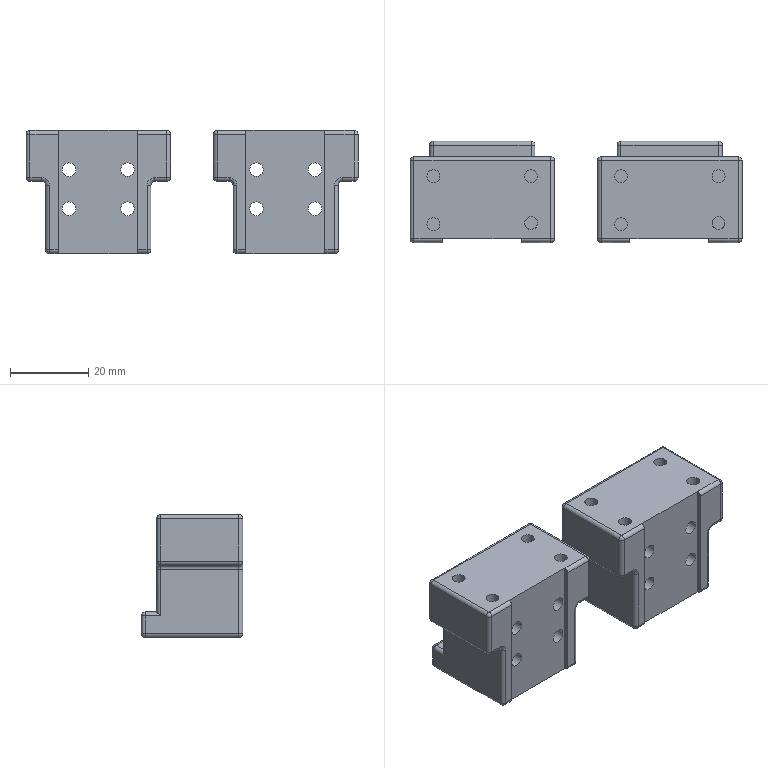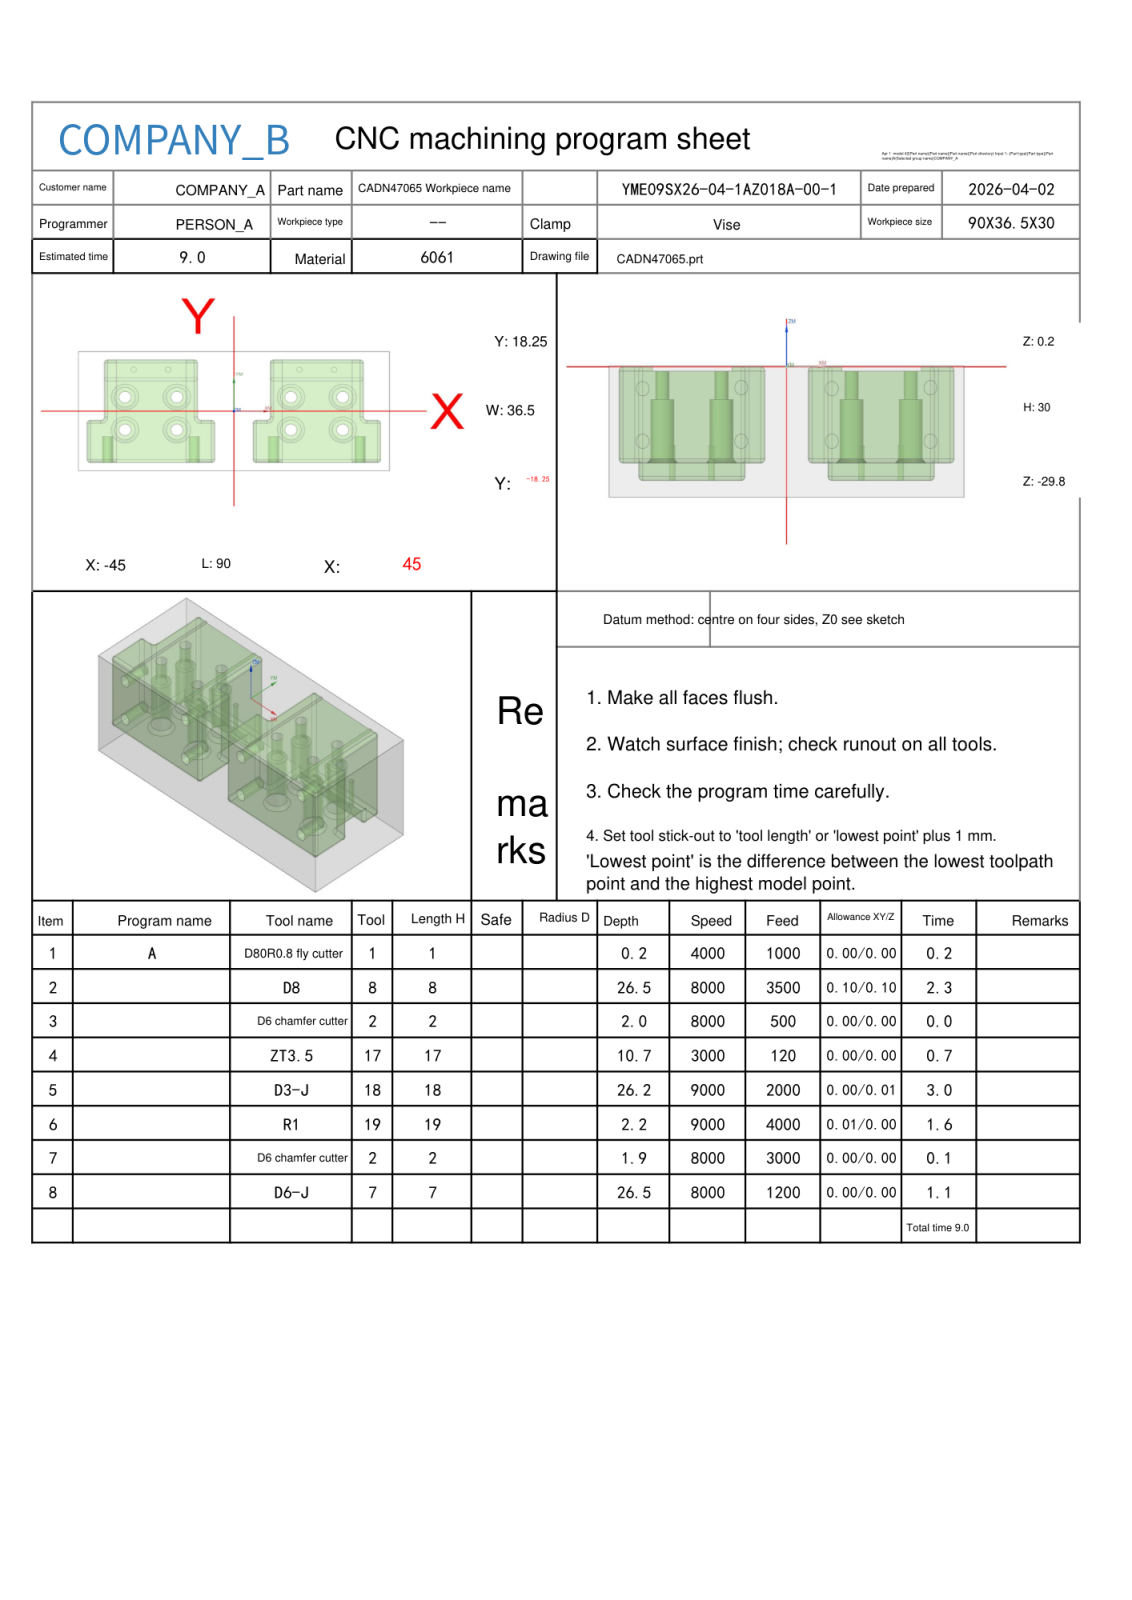NC program | NX | posted by the shop | part box 85 x 26 x 31.5 mm
Lines 1 to 33 of 17928:
%
O0001
(Machine time: 10.62 MIN)
(===Total Tool:7===)
(T1=D80R0.8 fly cutter D=80.  R=0.8  D-  H01 Z=0.    )
(T8=D8      D=8.   R=0.   D-  H08 Z=-26.3 )
(T2=D6 chamfer cutter   D=6.   R=0.   D-  H02 Z=-1.8  )
(T17=ZT3.5  D=3.5  DR_a=118 D-  H17 Z=-10.54)
(T18=D3-J   D=3.   R=0.   D-  H18 Z=-25.95)
(T19=R1     D=2.   R=1.   D-  H19 Z=-2.   )
(T7=D6-J    D=6.   R=0.   D7  H07 Z=-26.3 )
G80 G90 G17 G49 G40
G91 G28 Z0
M01
N1 T01 M06
(D80R0.8 fly cutter  D=80. R=0.8 H=01 ce=0.00 di=0.00)
G00 G90 G54 X-87.5 Y0.0 M03 S4000
G43 H01 Z20.
M08
Z2.
G01 Z0.0 F1000.
X-82.5
X82.5
X87.5
Z2.
G00 Z20.
G91 G28 Z0.0
M05
M09
G91 G28 Z0.0
M01